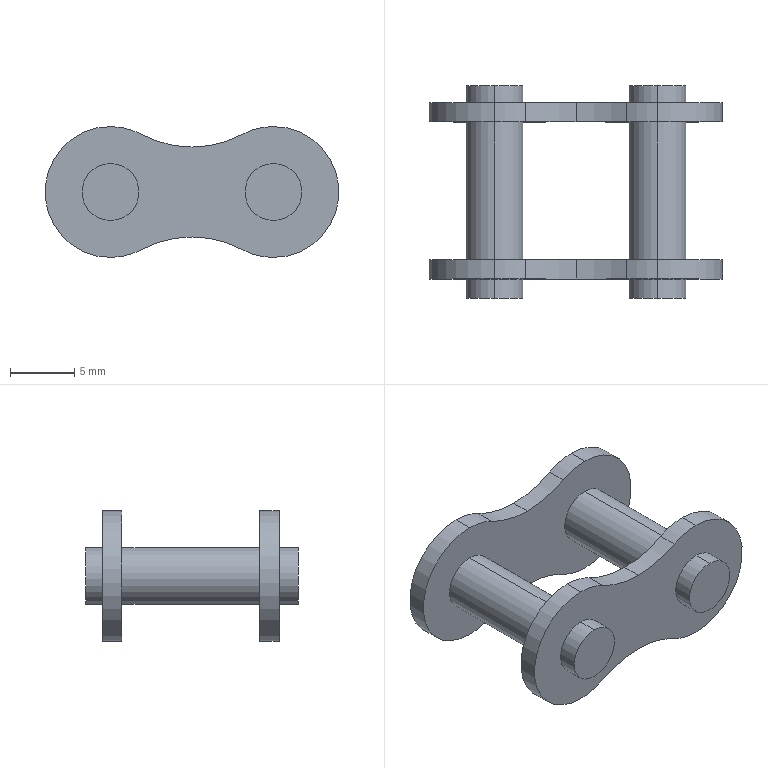Part | SolidWorks | features BaseBody 1 | 1 solid | 38 faces | box 22.9 x 16.575 x 10.2 mm | volume 988.18 mm3 | cylinder 30 | plane 8 | commonest cylinder face diameters 4.44 x12 10.2 x12 16.655 x6
STEP:
#1=CARTESIAN_POINT('',(-416.726,-324.843,-253.348));
#2=VERTEX_POINT('',#1);
#3=CARTESIAN_POINT('',(-416.726,-324.843,-257.788));
#4=VERTEX_POINT('',#3);
#5=CARTESIAN_POINT('',(-416.726,-324.843,-255.568));
#6=DIRECTION('',(-0.000000001,-1.,-0.000000001));
#7=DIRECTION('',(-0.000000001,0.000000001,-1.));
#8=AXIS2_PLACEMENT_3D('',#5,#6,#7);
#9=CIRCLE('',#8,2.22);
#10=EDGE_CURVE('',#2,#4,#9,.T.);
#11=ORIENTED_EDGE('',*,*,#10,.F.);
#12=CARTESIAN_POINT('',(-416.726,-323.343,-253.348));
#13=VERTEX_POINT('',#12);
#14=CARTESIAN_POINT('',(-416.726,-328.343,-253.348));
#15=DIRECTION('',(0.000000001,1.,0.000000001));
#16=VECTOR('',#15,1000.);
#17=LINE('',#14,#16);
#18=EDGE_CURVE('',#2,#13,#17,.T.);
#19=ORIENTED_EDGE('',*,*,#18,.T.);
#20=CARTESIAN_POINT('',(-416.726,-323.343,-257.788));
#21=VERTEX_POINT('',#20);
#22=CARTESIAN_POINT('',(-416.726,-323.343,-255.568));
#23=DIRECTION('',(0.000000001,1.,0.000000001));
#24=DIRECTION('',(-0.000000001,0.000000001,-1.));
#25=AXIS2_PLACEMENT_3D('',#22,#23,#24);
#26=CIRCLE('',#25,2.22);
#27=EDGE_CURVE('',#21,#13,#26,.T.);
#28=ORIENTED_EDGE('',*,*,#27,.F.);
#29=CARTESIAN_POINT('',(-416.726,-328.343,-257.788));
#30=DIRECTION('',(0.000000001,1.,0.000000001));
#31=VECTOR('',#30,1000.);
#32=LINE('',#29,#31);
#33=EDGE_CURVE('',#4,#21,#32,.T.);
#34=ORIENTED_EDGE('',*,*,#33,.F.);
#35=EDGE_LOOP('',(#11,#19,#28,#34));
#36=FACE_OUTER_BOUND('',#35,.T.);
#37=CARTESIAN_POINT('',(-416.726,-328.343,-255.568));
#38=DIRECTION('',(0.000000001,1.,0.000000001));
#39=DIRECTION('',(-0.000000001,0.000000001,-1.));
#40=AXIS2_PLACEMENT_3D('',#37,#38,#39);
#41=CYLINDRICAL_SURFACE('',#40,2.22);
#42=ADVANCED_FACE('',(#36),#41,.T.);
#43=CARTESIAN_POINT('',(-429.426,-324.843,-253.348));
#44=VERTEX_POINT('',#43);
#45=CARTESIAN_POINT('',(-429.426,-324.843,-257.788));
#46=VERTEX_POINT('',#45);
#47=CARTESIAN_POINT('',(-429.426,-324.843,-255.568));
#48=DIRECTION('',(-0.000000001,-1.,-0.000000001));
#49=DIRECTION('',(-0.000000001,0.000000001,-1.));
#50=AXIS2_PLACEMENT_3D('',#47,#48,#49);
#51=CIRCLE('',#50,2.22);
#52=EDGE_CURVE('',#44,#46,#51,.T.);
#53=ORIENTED_EDGE('',*,*,#52,.F.);
#54=CARTESIAN_POINT('',(-429.426,-323.343,-253.348));
#55=VERTEX_POINT('',#54);
#56=CARTESIAN_POINT('',(-429.426,-328.343,-253.348));
#57=DIRECTION('',(0.000000001,1.,0.000000001));
#58=VECTOR('',#57,1000.);
#59=LINE('',#56,#58);
#60=EDGE_CURVE('',#44,#55,#59,.T.);
#61=ORIENTED_EDGE('',*,*,#60,.T.);
#62=CARTESIAN_POINT('',(-429.426,-323.343,-257.788));
#63=VERTEX_POINT('',#62);
#64=CARTESIAN_POINT('',(-429.426,-323.343,-255.568));
#65=DIRECTION('',(0.000000001,1.,0.000000001));
#66=DIRECTION('',(-0.000000001,0.000000001,-1.));
#67=AXIS2_PLACEMENT_3D('',#64,#65,#66);
#68=CIRCLE('',#67,2.22);
#69=EDGE_CURVE('',#63,#55,#68,.T.);
#70=ORIENTED_EDGE('',*,*,#69,.F.);
#71=CARTESIAN_POINT('',(-429.426,-328.343,-257.788));
#72=DIRECTION('',(0.000000001,1.,0.000000001));
#73=VECTOR('',#72,1000.);
#74=LINE('',#71,#73);
#75=EDGE_CURVE('',#46,#63,#74,.T.);
#76=ORIENTED_EDGE('',*,*,#75,.F.);
#77=EDGE_LOOP('',(#53,#61,#70,#76));
#78=FACE_OUTER_BOUND('',#77,.T.);
#79=CARTESIAN_POINT('',(-429.426,-328.343,-255.568));
#80=DIRECTION('',(0.000000001,1.,0.000000001));
#81=DIRECTION('',(-0.000000001,0.000000001,-1.));
#82=AXIS2_PLACEMENT_3D('',#79,#80,#81);
#83=CYLINDRICAL_SURFACE('',#82,2.22);
#84=ADVANCED_FACE('',(#78),#83,.T.);
#85=CARTESIAN_POINT('',(-416.726,-309.593,-257.788));
#86=VERTEX_POINT('',#85);
#87=CARTESIAN_POINT('',(-416.726,-309.593,-253.348));
#88=VERTEX_POINT('',#87);
#89=CARTESIAN_POINT('',(-416.726,-309.593,-255.568));
#90=DIRECTION('',(0.000000001,1.,0.000000001));
#91=DIRECTION('',(-0.000000001,0.000000001,-1.));
#92=AXIS2_PLACEMENT_3D('',#89,#90,#91);
#93=CIRCLE('',#92,2.22);
#94=EDGE_CURVE('',#86,#88,#93,.T.);
#95=ORIENTED_EDGE('',*,*,#94,.T.);
#96=CARTESIAN_POINT('',(-416.726,-308.268,-253.348));
#97=VERTEX_POINT('',#96);
#98=CARTESIAN_POINT('',(-416.726,-328.343,-253.348));
#99=DIRECTION('',(0.000000001,1.,0.000000001));
#100=VECTOR('',#99,1000.);
#101=LINE('',#98,#100);
#102=EDGE_CURVE('',#88,#97,#101,.T.);
#103=ORIENTED_EDGE('',*,*,#102,.T.);
#104=CARTESIAN_POINT('',(-416.726,-308.268,-257.788));
#105=VERTEX_POINT('',#104);
#106=CARTESIAN_POINT('',(-416.726,-308.268,-255.568));
#107=DIRECTION('',(-0.000000001,-1.,-0.000000001));
#108=DIRECTION('',(-0.000000001,0.000000001,-1.));
#109=AXIS2_PLACEMENT_3D('',#106,#107,#108);
#110=CIRCLE('',#109,2.22);
#111=EDGE_CURVE('',#97,#105,#110,.T.);
#112=ORIENTED_EDGE('',*,*,#111,.T.);
#113=CARTESIAN_POINT('',(-416.726,-328.343,-257.788));
#114=DIRECTION('',(0.000000001,1.,0.000000001));
#115=VECTOR('',#114,1000.);
#116=LINE('',#113,#115);
#117=EDGE_CURVE('',#86,#105,#116,.T.);
#118=ORIENTED_EDGE('',*,*,#117,.F.);
#119=EDGE_LOOP('',(#95,#103,#112,#118));
#120=FACE_OUTER_BOUND('',#119,.T.);
#121=CARTESIAN_POINT('',(-416.726,-328.343,-255.568));
#122=DIRECTION('',(0.000000001,1.,0.000000001));
#123=DIRECTION('',(-0.000000001,0.000000001,-1.));
#124=AXIS2_PLACEMENT_3D('',#121,#122,#123);
#125=CYLINDRICAL_SURFACE('',#124,2.22);
#126=ADVANCED_FACE('',(#120),#125,.T.);
#127=CARTESIAN_POINT('',(-429.426,-321.843,-257.788));
#128=VERTEX_POINT('',#127);
#129=CARTESIAN_POINT('',(-429.426,-321.843,-253.348));
#130=VERTEX_POINT('',#129);
#131=CARTESIAN_POINT('',(-429.426,-321.843,-255.568));
#132=DIRECTION('',(0.000000001,1.,0.000000001));
#133=DIRECTION('',(-0.000000001,0.000000001,-1.));
#134=AXIS2_PLACEMENT_3D('',#131,#132,#133);
#135=CIRCLE('',#134,2.22);
#136=EDGE_CURVE('',#128,#130,#135,.T.);
#137=ORIENTED_EDGE('',*,*,#136,.T.);
#138=CARTESIAN_POINT('',(-429.426,-311.093,-253.348));
#139=VERTEX_POINT('',#138);
#140=CARTESIAN_POINT('',(-429.426,-328.343,-253.348));
#141=DIRECTION('',(0.000000001,1.,0.000000001));
#142=VECTOR('',#141,1000.);
#143=LINE('',#140,#142);
#144=EDGE_CURVE('',#130,#139,#143,.T.);
#145=ORIENTED_EDGE('',*,*,#144,.T.);
#146=CARTESIAN_POINT('',(-429.426,-311.093,-257.788));
#147=VERTEX_POINT('',#146);
#148=CARTESIAN_POINT('',(-429.426,-311.093,-255.568));
#149=DIRECTION('',(0.000000001,1.,0.000000001));
#150=DIRECTION('',(1.,-0.000000001,-0.000000001));
#151=AXIS2_PLACEMENT_3D('',#148,#149,#150);
#152=CIRCLE('',#151,2.22);
#153=EDGE_CURVE('',#147,#139,#152,.T.);
#154=ORIENTED_EDGE('',*,*,#153,.F.);
#155=CARTESIAN_POINT('',(-429.426,-328.343,-257.788));
#156=DIRECTION('',(0.000000001,1.,0.000000001));
#157=VECTOR('',#156,1000.);
#158=LINE('',#155,#157);
#159=EDGE_CURVE('',#128,#147,#158,.T.);
#160=ORIENTED_EDGE('',*,*,#159,.F.);
#161=EDGE_LOOP('',(#137,#145,#154,#160));
#162=FACE_OUTER_BOUND('',#161,.T.);
#163=CARTESIAN_POINT('',(-429.426,-328.343,-255.568));
#164=DIRECTION('',(0.000000001,1.,0.000000001));
#165=DIRECTION('',(-0.000000001,0.000000001,-1.));
#166=AXIS2_PLACEMENT_3D('',#163,#164,#165);
#167=CYLINDRICAL_SURFACE('',#166,2.22);
#168=ADVANCED_FACE('',(#162),#167,.T.);
#169=CARTESIAN_POINT('',(-429.426,-309.593,-253.348));
#170=VERTEX_POINT('',#169);
#171=CARTESIAN_POINT('',(-429.426,-309.593,-257.788));
#172=VERTEX_POINT('',#171);
#173=CARTESIAN_POINT('',(-429.426,-309.593,-255.568));
#174=DIRECTION('',(-0.000000001,-1.,-0.000000001));
#175=DIRECTION('',(-0.000000001,0.000000001,-1.));
#176=AXIS2_PLACEMENT_3D('',#173,#174,#175);
#177=CIRCLE('',#176,2.22);
#178=EDGE_CURVE('',#170,#172,#177,.T.);
#179=ORIENTED_EDGE('',*,*,#178,.F.);
#180=CARTESIAN_POINT('',(-429.426,-308.268,-253.348));
#181=VERTEX_POINT('',#180);
#182=CARTESIAN_POINT('',(-429.426,-328.343,-253.348));
#183=DIRECTION('',(0.000000001,1.,0.000000001));
#184=VECTOR('',#183,1000.);
#185=LINE('',#182,#184);
#186=EDGE_CURVE('',#170,#181,#185,.T.);
#187=ORIENTED_EDGE('',*,*,#186,.T.);
#188=CARTESIAN_POINT('',(-429.426,-308.268,-257.788));
#189=VERTEX_POINT('',#188);
#190=CARTESIAN_POINT('',(-429.426,-308.268,-255.568));
#191=DIRECTION('',(-0.000000001,-1.,-0.000000001));
#192=DIRECTION('',(-0.000000001,0.000000001,-1.));
#193=AXIS2_PLACEMENT_3D('',#190,#191,#192);
#194=CIRCLE('',#193,2.22);
#195=EDGE_CURVE('',#181,#189,#194,.T.);
#196=ORIENTED_EDGE('',*,*,#195,.T.);
#197=CARTESIAN_POINT('',(-429.426,-328.343,-257.788));
#198=DIRECTION('',(0.000000001,1.,0.000000001));
#199=VECTOR('',#198,1000.);
#200=LINE('',#197,#199);
#201=EDGE_CURVE('',#172,#189,#200,.T.);
#202=ORIENTED_EDGE('',*,*,#201,.F.);
#203=EDGE_LOOP('',(#179,#187,#196,#202));
#204=FACE_OUTER_BOUND('',#203,.T.);
#205=CARTESIAN_POINT('',(-429.426,-328.343,-255.568));
#206=DIRECTION('',(0.000000001,1.,0.000000001));
#207=DIRECTION('',(-0.000000001,0.000000001,-1.));
#208=AXIS2_PLACEMENT_3D('',#205,#206,#207);
#209=CYLINDRICAL_SURFACE('',#208,2.22);
#210=ADVANCED_FACE('',(#204),#209,.T.);
#211=CARTESIAN_POINT('',(-423.076,-311.093,-252.065));
#212=VERTEX_POINT('',#211);
#213=CARTESIAN_POINT('',(-427.014,-311.093,-251.075));
#214=VERTEX_POINT('',#213);
#215=CARTESIAN_POINT('',(-423.076,-311.093,-243.737));
#216=DIRECTION('',(0.000000001,1.,0.000000001));
#217=DIRECTION('',(1.,-0.000000001,-0.000000001));
#218=AXIS2_PLACEMENT_3D('',#215,#216,#217);
#219=CIRCLE('',#218,8.327);
#220=EDGE_CURVE('',#212,#214,#219,.T.);
#221=ORIENTED_EDGE('',*,*,#220,.F.);
#222=CARTESIAN_POINT('',(-423.076,-309.593,-252.065));
#223=VERTEX_POINT('',#222);
#224=CARTESIAN_POINT('',(-423.076,-311.093,-252.065));
#225=DIRECTION('',(0.000000001,1.,0.000000001));
#226=VECTOR('',#225,1000.);
#227=LINE('',#224,#226);
#228=EDGE_CURVE('',#212,#223,#227,.T.);
#229=ORIENTED_EDGE('',*,*,#228,.T.);
#230=CARTESIAN_POINT('',(-427.014,-309.593,-251.075));
#231=VERTEX_POINT('',#230);
#232=CARTESIAN_POINT('',(-423.076,-309.593,-243.737));
#233=DIRECTION('',(0.000000001,1.,0.000000001));
#234=DIRECTION('',(1.,-0.000000001,-0.000000001));
#235=AXIS2_PLACEMENT_3D('',#232,#233,#234);
#236=CIRCLE('',#235,8.327);
#237=EDGE_CURVE('',#223,#231,#236,.T.);
#238=ORIENTED_EDGE('',*,*,#237,.T.);
#239=CARTESIAN_POINT('',(-427.014,-311.093,-251.075));
#240=DIRECTION('',(0.000000001,1.,0.000000001));
#241=VECTOR('',#240,1000.);
#242=LINE('',#239,#241);
#243=EDGE_CURVE('',#214,#231,#242,.T.);
#244=ORIENTED_EDGE('',*,*,#243,.F.);
#245=EDGE_LOOP('',(#221,#229,#238,#244));
#246=FACE_OUTER_BOUND('',#245,.T.);
#247=CARTESIAN_POINT('',(-423.076,-311.093,-243.737));
#248=DIRECTION('',(0.000000001,1.,0.000000001));
#249=DIRECTION('',(-0.000000001,0.000000001,-1.));
#250=AXIS2_PLACEMENT_3D('',#247,#248,#249);
#251=CYLINDRICAL_SURFACE('',#250,8.327);
#252=ADVANCED_FACE('',(#246),#251,.F.);
#253=CARTESIAN_POINT('',(-416.726,-311.093,-250.468));
#254=VERTEX_POINT('',#253);
#255=CARTESIAN_POINT('',(-419.115,-311.093,-251.063));
#256=VERTEX_POINT('',#255);
#257=CARTESIAN_POINT('',(-416.726,-311.093,-255.568));
#258=DIRECTION('',(-0.000000001,-1.,-0.000000001));
#259=DIRECTION('',(1.,-0.000000001,-0.000000001));
#260=AXIS2_PLACEMENT_3D('',#257,#258,#259);
#261=CIRCLE('',#260,5.1);
#262=EDGE_CURVE('',#254,#256,#261,.T.);
#263=ORIENTED_EDGE('',*,*,#262,.F.);
#264=CARTESIAN_POINT('',(-416.726,-309.593,-250.468));
#265=VERTEX_POINT('',#264);
#266=CARTESIAN_POINT('',(-416.726,-311.093,-250.468));
#267=DIRECTION('',(0.000000001,1.,0.000000001));
#268=VECTOR('',#267,1000.);
#269=LINE('',#266,#268);
#270=EDGE_CURVE('',#254,#265,#269,.T.);
#271=ORIENTED_EDGE('',*,*,#270,.T.);
#272=CARTESIAN_POINT('',(-419.115,-309.593,-251.063));
#273=VERTEX_POINT('',#272);
#274=CARTESIAN_POINT('',(-416.726,-309.593,-255.568));
#275=DIRECTION('',(-0.000000001,-1.,-0.000000001));
#276=DIRECTION('',(1.,-0.000000001,-0.000000001));
#277=AXIS2_PLACEMENT_3D('',#274,#275,#276);
#278=CIRCLE('',#277,5.1);
#279=EDGE_CURVE('',#265,#273,#278,.T.);
#280=ORIENTED_EDGE('',*,*,#279,.T.);
#281=CARTESIAN_POINT('',(-419.115,-311.093,-251.063));
#282=DIRECTION('',(0.000000001,1.,0.000000001));
#283=VECTOR('',#282,1000.);
#284=LINE('',#281,#283);
#285=EDGE_CURVE('',#256,#273,#284,.T.);
#286=ORIENTED_EDGE('',*,*,#285,.F.);
#287=EDGE_LOOP('',(#263,#271,#280,#286));
#288=FACE_OUTER_BOUND('',#287,.T.);
#289=CARTESIAN_POINT('',(-416.726,-311.093,-255.568));
#290=DIRECTION('',(0.000000001,1.,0.000000001));
#291=DIRECTION('',(-0.000000001,0.000000001,-1.));
#292=AXIS2_PLACEMENT_3D('',#289,#290,#291);
#293=CYLINDRICAL_SURFACE('',#292,5.1);
#294=ADVANCED_FACE('',(#288),#293,.T.);
#295=ORIENTED_EDGE('',*,*,#270,.F.);
#296=CARTESIAN_POINT('',(-416.726,-311.093,-260.668));
#297=VERTEX_POINT('',#296);
#298=CARTESIAN_POINT('',(-416.726,-311.093,-255.568));
#299=DIRECTION('',(-0.000000001,-1.,-0.000000001));
#300=DIRECTION('',(1.,-0.000000001,-0.000000001));
#301=AXIS2_PLACEMENT_3D('',#298,#299,#300);
#302=CIRCLE('',#301,5.1);
#303=EDGE_CURVE('',#297,#254,#302,.T.);
#304=ORIENTED_EDGE('',*,*,#303,.F.);
#305=CARTESIAN_POINT('',(-416.726,-309.593,-260.668));
#306=VERTEX_POINT('',#305);
#307=CARTESIAN_POINT('',(-416.726,-311.093,-260.668));
#308=DIRECTION('',(0.000000001,1.,0.000000001));
#309=VECTOR('',#308,1000.);
#310=LINE('',#307,#309);
#311=EDGE_CURVE('',#297,#306,#310,.T.);
#312=ORIENTED_EDGE('',*,*,#311,.T.);
#313=CARTESIAN_POINT('',(-416.726,-309.593,-255.568));
#314=DIRECTION('',(-0.000000001,-1.,-0.000000001));
#315=DIRECTION('',(1.,-0.000000001,-0.000000001));
#316=AXIS2_PLACEMENT_3D('',#313,#314,#315);
#317=CIRCLE('',#316,5.1);
#318=EDGE_CURVE('',#306,#265,#317,.T.);
#319=ORIENTED_EDGE('',*,*,#318,.T.);
#320=EDGE_LOOP('',(#295,#304,#312,#319));
#321=FACE_OUTER_BOUND('',#320,.T.);
#322=CARTESIAN_POINT('',(-416.726,-311.093,-255.568));
#323=DIRECTION('',(0.000000001,1.,0.000000001));
#324=DIRECTION('',(-0.000000001,0.000000001,-1.));
#325=AXIS2_PLACEMENT_3D('',#322,#323,#324);
#326=CYLINDRICAL_SURFACE('',#325,5.1);
#327=ADVANCED_FACE('',(#321),#326,.T.);
#328=CARTESIAN_POINT('',(-429.426,-311.093,-250.468));
#329=VERTEX_POINT('',#328);
#330=CARTESIAN_POINT('',(-429.426,-311.093,-260.668));
#331=VERTEX_POINT('',#330);
#332=CARTESIAN_POINT('',(-429.426,-311.093,-255.568));
#333=DIRECTION('',(-0.000000001,-1.,-0.000000001));
#334=DIRECTION('',(1.,-0.000000001,-0.000000001));
#335=AXIS2_PLACEMENT_3D('',#332,#333,#334);
#336=CIRCLE('',#335,5.1);
#337=EDGE_CURVE('',#329,#331,#336,.T.);
#338=ORIENTED_EDGE('',*,*,#337,.F.);
#339=CARTESIAN_POINT('',(-429.426,-309.593,-250.468));
#340=VERTEX_POINT('',#339);
#341=CARTESIAN_POINT('',(-429.426,-311.093,-250.468));
#342=DIRECTION('',(0.000000001,1.,0.000000001));
#343=VECTOR('',#342,1000.);
#344=LINE('',#341,#343);
#345=EDGE_CURVE('',#329,#340,#344,.T.);
#346=ORIENTED_EDGE('',*,*,#345,.T.);
#347=CARTESIAN_POINT('',(-429.426,-309.593,-260.668));
#348=VERTEX_POINT('',#347);
#349=CARTESIAN_POINT('',(-429.426,-309.593,-255.568));
#350=DIRECTION('',(-0.000000001,-1.,-0.000000001));
#351=DIRECTION('',(1.,-0.000000001,-0.000000001));
#352=AXIS2_PLACEMENT_3D('',#349,#350,#351);
#353=CIRCLE('',#352,5.1);
#354=EDGE_CURVE('',#340,#348,#353,.T.);
#355=ORIENTED_EDGE('',*,*,#354,.T.);
#356=CARTESIAN_POINT('',(-429.426,-311.093,-260.668));
#357=DIRECTION('',(0.000000001,1.,0.000000001));
#358=VECTOR('',#357,1000.);
#359=LINE('',#356,#358);
#360=EDGE_CURVE('',#331,#348,#359,.T.);
#361=ORIENTED_EDGE('',*,*,#360,.F.);
#362=EDGE_LOOP('',(#338,#346,#355,#361));
#363=FACE_OUTER_BOUND('',#362,.T.);
#364=CARTESIAN_POINT('',(-429.426,-311.093,-255.568));
#365=DIRECTION('',(0.000000001,1.,0.000000001));
#366=DIRECTION('',(-0.000000001,0.000000001,-1.));
#367=AXIS2_PLACEMENT_3D('',#364,#365,#366);
#368=CYLINDRICAL_SURFACE('',#367,5.1);
#369=ADVANCED_FACE('',(#363),#368,.T.);
#370=CARTESIAN_POINT('',(-427.014,-311.093,-260.062));
#371=VERTEX_POINT('',#370);
#372=CARTESIAN_POINT('',(-429.426,-311.093,-255.568));
#373=DIRECTION('',(-0.000000001,-1.,-0.000000001));
#374=DIRECTION('',(1.,-0.000000001,-0.000000001));
#375=AXIS2_PLACEMENT_3D('',#372,#373,#374);
#376=CIRCLE('',#375,5.1);
#377=EDGE_CURVE('',#331,#371,#376,.T.);
#378=ORIENTED_EDGE('',*,*,#377,.F.);
#379=ORIENTED_EDGE('',*,*,#360,.T.);
#380=CARTESIAN_POINT('',(-427.014,-309.593,-260.062));
#381=VERTEX_POINT('',#380);
#382=CARTESIAN_POINT('',(-429.426,-309.593,-255.568));
#383=DIRECTION('',(-0.000000001,-1.,-0.000000001));
#384=DIRECTION('',(1.,-0.000000001,-0.000000001));
#385=AXIS2_PLACEMENT_3D('',#382,#383,#384);
#386=CIRCLE('',#385,5.1);
#387=EDGE_CURVE('',#348,#381,#386,.T.);
#388=ORIENTED_EDGE('',*,*,#387,.T.);
#389=CARTESIAN_POINT('',(-427.014,-311.093,-260.062));
#390=DIRECTION('',(0.000000001,1.,0.000000001));
#391=VECTOR('',#390,1000.);
#392=LINE('',#389,#391);
#393=EDGE_CURVE('',#371,#381,#392,.T.);
#394=ORIENTED_EDGE('',*,*,#393,.F.);
#395=EDGE_LOOP('',(#378,#379,#388,#394));
#396=FACE_OUTER_BOUND('',#395,.T.);
#397=CARTESIAN_POINT('',(-429.426,-311.093,-255.568));
#398=DIRECTION('',(0.000000001,1.,0.000000001));
#399=DIRECTION('',(-0.000000001,0.000000001,-1.));
#400=AXIS2_PLACEMENT_3D('',#397,#398,#399);
#401=CYLINDRICAL_SURFACE('',#400,5.1);
#402=ADVANCED_FACE('',(#396),#401,.T.);
#403=CARTESIAN_POINT('',(-416.726,-321.843,-257.788));
#404=VERTEX_POINT('',#403);
#405=CARTESIAN_POINT('',(-416.726,-321.843,-253.348));
#406=VERTEX_POINT('',#405);
#407=CARTESIAN_POINT('',(-416.726,-321.843,-255.568));
#408=DIRECTION('',(0.000000001,1.,0.000000001));
#409=DIRECTION('',(-0.000000001,0.000000001,-1.));
#410=AXIS2_PLACEMENT_3D('',#407,#408,#409);
#411=CIRCLE('',#410,2.22);
#412=EDGE_CURVE('',#404,#406,#411,.T.);
#413=ORIENTED_EDGE('',*,*,#412,.T.);
#414=CARTESIAN_POINT('',(-416.726,-311.093,-253.348));
#415=VERTEX_POINT('',#414);
#416=CARTESIAN_POINT('',(-416.726,-328.343,-253.348));
#417=DIRECTION('',(0.000000001,1.,0.000000001));
#418=VECTOR('',#417,1000.);
#419=LINE('',#416,#418);
#420=EDGE_CURVE('',#406,#415,#419,.T.);
#421=ORIENTED_EDGE('',*,*,#420,.T.);
#422=CARTESIAN_POINT('',(-416.726,-311.093,-257.788));
#423=VERTEX_POINT('',#422);
#424=CARTESIAN_POINT('',(-416.726,-311.093,-255.568));
#425=DIRECTION('',(0.000000001,1.,0.000000001));
#426=DIRECTION('',(1.,-0.000000001,-0.000000001));
#427=AXIS2_PLACEMENT_3D('',#424,#425,#426);
#428=CIRCLE('',#427,2.22);
#429=EDGE_CURVE('',#423,#415,#428,.T.);
#430=ORIENTED_EDGE('',*,*,#429,.F.);
#431=CARTESIAN_POINT('',(-416.726,-328.343,-257.788));
#432=DIRECTION('',(0.000000001,1.,0.000000001));
#433=VECTOR('',#432,1000.);
#434=LINE('',#431,#433);
#435=EDGE_CURVE('',#404,#423,#434,.T.);
#436=ORIENTED_EDGE('',*,*,#435,.F.);
#437=EDGE_LOOP('',(#413,#421,#430,#436));
#438=FACE_OUTER_BOUND('',#437,.T.);
#439=CARTESIAN_POINT('',(-416.726,-328.343,-255.568));
#440=DIRECTION('',(0.000000001,1.,0.000000001));
#441=DIRECTION('',(-0.000000001,0.000000001,-1.));
#442=AXIS2_PLACEMENT_3D('',#439,#440,#441);
#443=CYLINDRICAL_SURFACE('',#442,2.22);
#444=ADVANCED_FACE('',(#438),#443,.T.);
#445=CARTESIAN_POINT('',(-429.426,-323.343,-250.468));
#446=VERTEX_POINT('',#445);
#447=CARTESIAN_POINT('',(-429.426,-323.343,-260.668));
#448=VERTEX_POINT('',#447);
#449=CARTESIAN_POINT('',(-429.426,-323.343,-255.568));
#450=DIRECTION('',(-0.000000001,-1.,-0.000000001));
#451=DIRECTION('',(-0.000000001,0.000000001,-1.));
#452=AXIS2_PLACEMENT_3D('',#449,#450,#451);
#453=CIRCLE('',#452,5.1);
#454=EDGE_CURVE('',#446,#448,#453,.T.);
#455=ORIENTED_EDGE('',*,*,#454,.F.);
#456=CARTESIAN_POINT('',(-429.426,-321.843,-250.468));
#457=VERTEX_POINT('',#456);
#458=CARTESIAN_POINT('',(-429.426,-324.843,-250.468));
#459=DIRECTION('',(0.000000001,1.,0.000000001));
#460=VECTOR('',#459,1000.);
#461=LINE('',#458,#460);
#462=EDGE_CURVE('',#446,#457,#461,.T.);
#463=ORIENTED_EDGE('',*,*,#462,.T.);
#464=CARTESIAN_POINT('',(-429.426,-321.843,-260.668));
#465=VERTEX_POINT('',#464);
#466=CARTESIAN_POINT('',(-429.426,-321.843,-255.568));
#467=DIRECTION('',(-0.000000001,-1.,-0.000000001));
#468=DIRECTION('',(1.,-0.000000001,-0.000000001));
#469=AXIS2_PLACEMENT_3D('',#466,#467,#468);
#470=CIRCLE('',#469,5.1);
#471=EDGE_CURVE('',#457,#465,#470,.T.);
#472=ORIENTED_EDGE('',*,*,#471,.T.);
#473=CARTESIAN_POINT('',(-429.426,-324.843,-260.668));
#474=DIRECTION('',(0.000000001,1.,0.000000001));
#475=VECTOR('',#474,1000.);
#476=LINE('',#473,#475);
#477=EDGE_CURVE('',#448,#465,#476,.T.);
#478=ORIENTED_EDGE('',*,*,#477,.F.);
#479=EDGE_LOOP('',(#455,#463,#472,#478));
#480=FACE_OUTER_BOUND('',#479,.T.);
#481=CARTESIAN_POINT('',(-429.426,-324.843,-255.568));
#482=DIRECTION('',(0.000000001,1.,0.000000001));
#483=DIRECTION('',(-0.000000001,0.000000001,-1.));
#484=AXIS2_PLACEMENT_3D('',#481,#482,#483);
#485=CYLINDRICAL_SURFACE('',#484,5.1);
#486=ADVANCED_FACE('',(#480),#485,.T.);
#487=CARTESIAN_POINT('',(-427.014,-323.343,-260.062));
#488=VERTEX_POINT('',#487);
#489=CARTESIAN_POINT('',(-429.426,-323.343,-255.568));
#490=DIRECTION('',(-0.000000001,-1.,-0.000000001));
#491=DIRECTION('',(-0.000000001,0.000000001,-1.));
#492=AXIS2_PLACEMENT_3D('',#489,#490,#491);
#493=CIRCLE('',#492,5.1);
#494=EDGE_CURVE('',#448,#488,#493,.T.);
#495=ORIENTED_EDGE('',*,*,#494,.F.);
#496=ORIENTED_EDGE('',*,*,#477,.T.);
#497=CARTESIAN_POINT('',(-427.014,-321.843,-260.062));
#498=VERTEX_POINT('',#497);
#499=CARTESIAN_POINT('',(-429.426,-321.843,-255.568));
#500=DIRECTION('',(-0.000000001,-1.,-0.000000001));
#501=DIRECTION('',(1.,-0.000000001,-0.000000001));
#502=AXIS2_PLACEMENT_3D('',#499,#500,#501);
#503=CIRCLE('',#502,5.1);
#504=EDGE_CURVE('',#465,#498,#503,.T.);
#505=ORIENTED_EDGE('',*,*,#504,.T.);
#506=CARTESIAN_POINT('',(-427.014,-324.843,-260.062));
#507=DIRECTION('',(0.000000001,1.,0.000000001));
#508=VECTOR('',#507,1000.);
#509=LINE('',#506,#508);
#510=EDGE_CURVE('',#488,#498,#509,.T.);
#511=ORIENTED_EDGE('',*,*,#510,.F.);
#512=EDGE_LOOP('',(#495,#496,#505,#511));
#513=FACE_OUTER_BOUND('',#512,.T.);
#514=CARTESIAN_POINT('',(-429.426,-324.843,-255.568));
#515=DIRECTION('',(0.000000001,1.,0.000000001));
#516=DIRECTION('',(-0.000000001,0.000000001,-1.));
#517=AXIS2_PLACEMENT_3D('',#514,#515,#516);
#518=CYLINDRICAL_SURFACE('',#517,5.1);
#519=ADVANCED_FACE('',(#513),#518,.T.);
#520=CARTESIAN_POINT('',(-416.726,-323.343,-250.468));
#521=VERTEX_POINT('',#520);
#522=CARTESIAN_POINT('',(-419.115,-323.343,-251.063));
#523=VERTEX_POINT('',#522);
#524=CARTESIAN_POINT('',(-416.726,-323.343,-255.568));
#525=DIRECTION('',(-0.000000001,-1.,-0.000000001));
#526=DIRECTION('',(-0.000000001,0.000000001,-1.));
#527=AXIS2_PLACEMENT_3D('',#524,#525,#526);
#528=CIRCLE('',#527,5.1);
#529=EDGE_CURVE('',#521,#523,#528,.T.);
#530=ORIENTED_EDGE('',*,*,#529,.F.);
#531=CARTESIAN_POINT('',(-416.726,-321.843,-250.468));
#532=VERTEX_POINT('',#531);
#533=CARTESIAN_POINT('',(-416.726,-324.843,-250.468));
#534=DIRECTION('',(0.000000001,1.,0.000000001));
#535=VECTOR('',#534,1000.);
#536=LINE('',#533,#535);
#537=EDGE_CURVE('',#521,#532,#536,.T.);
#538=ORIENTED_EDGE('',*,*,#537,.T.);
#539=CARTESIAN_POINT('',(-419.115,-321.843,-251.063));
#540=VERTEX_POINT('',#539);
#541=CARTESIAN_POINT('',(-416.726,-321.843,-255.568));
#542=DIRECTION('',(-0.000000001,-1.,-0.000000001));
#543=DIRECTION('',(1.,-0.000000001,-0.000000001));
#544=AXIS2_PLACEMENT_3D('',#541,#542,#543);
#545=CIRCLE('',#544,5.1);
#546=EDGE_CURVE('',#532,#540,#545,.T.);
#547=ORIENTED_EDGE('',*,*,#546,.T.);
#548=CARTESIAN_POINT('',(-419.115,-324.843,-251.063));
#549=DIRECTION('',(0.000000001,1.,0.000000001));
#550=VECTOR('',#549,1000.);
#551=LINE('',#548,#550);
#552=EDGE_CURVE('',#523,#540,#551,.T.);
#553=ORIENTED_EDGE('',*,*,#552,.F.);
#554=EDGE_LOOP('',(#530,#538,#547,#553));
#555=FACE_OUTER_BOUND('',#554,.T.);
#556=CARTESIAN_POINT('',(-416.726,-324.843,-255.568));
#557=DIRECTION('',(0.000000001,1.,0.000000001));
#558=DIRECTION('',(-0.000000001,0.000000001,-1.));
#559=AXIS2_PLACEMENT_3D('',#556,#557,#558);
#560=CYLINDRICAL_SURFACE('',#559,5.1);
#561=ADVANCED_FACE('',(#555),#560,.T.);
#562=ORIENTED_EDGE('',*,*,#537,.F.);
#563=CARTESIAN_POINT('',(-416.726,-323.343,-260.668));
#564=VERTEX_POINT('',#563);
#565=CARTESIAN_POINT('',(-416.726,-323.343,-255.568));
#566=DIRECTION('',(-0.000000001,-1.,-0.000000001));
#567=DIRECTION('',(-0.000000001,0.000000001,-1.));
#568=AXIS2_PLACEMENT_3D('',#565,#566,#567);
#569=CIRCLE('',#568,5.1);
#570=EDGE_CURVE('',#564,#521,#569,.T.);
#571=ORIENTED_EDGE('',*,*,#570,.F.);
#572=CARTESIAN_POINT('',(-416.726,-321.843,-260.668));
#573=VERTEX_POINT('',#572);
#574=CARTESIAN_POINT('',(-416.726,-324.843,-260.668));
#575=DIRECTION('',(0.000000001,1.,0.000000001));
#576=VECTOR('',#575,1000.);
#577=LINE('',#574,#576);
#578=EDGE_CURVE('',#564,#573,#577,.T.);
#579=ORIENTED_EDGE('',*,*,#578,.T.);
#580=CARTESIAN_POINT('',(-416.726,-321.843,-255.568));
#581=DIRECTION('',(-0.000000001,-1.,-0.000000001));
#582=DIRECTION('',(1.,-0.000000001,-0.000000001));
#583=AXIS2_PLACEMENT_3D('',#580,#581,#582);
#584=CIRCLE('',#583,5.1);
#585=EDGE_CURVE('',#573,#532,#584,.T.);
#586=ORIENTED_EDGE('',*,*,#585,.T.);
#587=EDGE_LOOP('',(#562,#571,#579,#586));
#588=FACE_OUTER_BOUND('',#587,.T.);
#589=CARTESIAN_POINT('',(-416.726,-324.843,-255.568));
#590=DIRECTION('',(0.000000001,1.,0.000000001));
#591=DIRECTION('',(-0.000000001,0.000000001,-1.));
#592=AXIS2_PLACEMENT_3D('',#589,#590,#591);
#593=CYLINDRICAL_SURFACE('',#592,5.1);
#594=ADVANCED_FACE('',(#588),#593,.T.);
#595=CARTESIAN_POINT('',(-423.076,-323.343,-252.065));
#596=VERTEX_POINT('',#595);
#597=CARTESIAN_POINT('',(-427.014,-323.343,-251.075));
#598=VERTEX_POINT('',#597);
#599=CARTESIAN_POINT('',(-423.076,-323.343,-243.737));
#600=DIRECTION('',(0.000000001,1.,0.000000001));
#601=DIRECTION('',(-0.000000001,0.000000001,-1.));
#602=AXIS2_PLACEMENT_3D('',#599,#600,#601);
#603=CIRCLE('',#602,8.327);
#604=EDGE_CURVE('',#596,#598,#603,.T.);
#605=ORIENTED_EDGE('',*,*,#604,.F.);
#606=CARTESIAN_POINT('',(-423.076,-321.843,-252.065));
#607=VERTEX_POINT('',#606);
#608=CARTESIAN_POINT('',(-423.076,-324.843,-252.065));
#609=DIRECTION('',(0.000000001,1.,0.000000001));
#610=VECTOR('',#609,1000.);
#611=LINE('',#608,#610);
#612=EDGE_CURVE('',#596,#607,#611,.T.);
#613=ORIENTED_EDGE('',*,*,#612,.T.);
#614=CARTESIAN_POINT('',(-427.014,-321.843,-251.075));
#615=VERTEX_POINT('',#614);
#616=CARTESIAN_POINT('',(-423.076,-321.843,-243.737));
#617=DIRECTION('',(0.000000001,1.,0.000000001));
#618=DIRECTION('',(1.,-0.000000001,-0.000000001));
#619=AXIS2_PLACEMENT_3D('',#616,#617,#618);
#620=CIRCLE('',#619,8.327);
#621=EDGE_CURVE('',#607,#615,#620,.T.);
#622=ORIENTED_EDGE('',*,*,#621,.T.);
#623=CARTESIAN_POINT('',(-427.014,-324.843,-251.075));
#624=DIRECTION('',(0.000000001,1.,0.000000001));
#625=VECTOR('',#624,1000.);
#626=LINE('',#623,#625);
#627=EDGE_CURVE('',#598,#615,#626,.T.);
#628=ORIENTED_EDGE('',*,*,#627,.F.);
#629=EDGE_LOOP('',(#605,#613,#622,#628));
#630=FACE_OUTER_BOUND('',#629,.T.);
#631=CARTESIAN_POINT('',(-423.076,-324.843,-243.737));
#632=DIRECTION('',(0.000000001,1.,0.000000001));
#633=DIRECTION('',(-0.000000001,0.000000001,-1.));
#634=AXIS2_PLACEMENT_3D('',#631,#632,#633);
#635=CYLINDRICAL_SURFACE('',#634,8.327);
#636=ADVANCED_FACE('',(#630),#635,.F.);
#637=ORIENTED_EDGE('',*,*,#612,.F.);
#638=CARTESIAN_POINT('',(-423.076,-323.343,-243.737));
#639=DIRECTION('',(0.000000001,1.,0.000000001));
#640=DIRECTION('',(-0.000000001,0.000000001,-1.));
#641=AXIS2_PLACEMENT_3D('',#638,#639,#640);
#642=CIRCLE('',#641,8.327);
#643=EDGE_CURVE('',#523,#596,#642,.T.);
#644=ORIENTED_EDGE('',*,*,#643,.F.);
#645=ORIENTED_EDGE('',*,*,#552,.T.);
#646=CARTESIAN_POINT('',(-423.076,-321.843,-243.737));
#647=DIRECTION('',(0.000000001,1.,0.000000001));
#648=DIRECTION('',(1.,-0.000000001,-0.000000001));
#649=AXIS2_PLACEMENT_3D('',#646,#647,#648);
#650=CIRCLE('',#649,8.327);
#651=EDGE_CURVE('',#540,#607,#650,.T.);
#652=ORIENTED_EDGE('',*,*,#651,.T.);
#653=EDGE_LOOP('',(#637,#644,#645,#652));
#654=FACE_OUTER_BOUND('',#653,.T.);
#655=CARTESIAN_POINT('',(-423.076,-324.843,-243.737));
#656=DIRECTION('',(0.000000001,1.,0.000000001));
#657=DIRECTION('',(-0.000000001,0.000000001,-1.));
#658=AXIS2_PLACEMENT_3D('',#655,#656,#657);
#659=CYLINDRICAL_SURFACE('',#658,8.327);
#660=ADVANCED_FACE('',(#654),#659,.F.);
#661=ORIENTED_EDGE('',*,*,#578,.F.);
#662=CARTESIAN_POINT('',(-419.115,-323.343,-260.074));
#663=VERTEX_POINT('',#662);
#664=CARTESIAN_POINT('',(-416.726,-323.343,-255.568));
#665=DIRECTION('',(-0.000000001,-1.,-0.000000001));
#666=DIRECTION('',(-0.000000001,0.000000001,-1.));
#667=AXIS2_PLACEMENT_3D('',#664,#665,#666);
#668=CIRCLE('',#667,5.1);
#669=EDGE_CURVE('',#663,#564,#668,.T.);
#670=ORIENTED_EDGE('',*,*,#669,.F.);
#671=CARTESIAN_POINT('',(-419.115,-321.843,-260.074));
#672=VERTEX_POINT('',#671);
#673=CARTESIAN_POINT('',(-419.115,-324.843,-260.074));
#674=DIRECTION('',(0.000000001,1.,0.000000001));
#675=VECTOR('',#674,1000.);
#676=LINE('',#673,#675);
#677=EDGE_CURVE('',#663,#672,#676,.T.);
#678=ORIENTED_EDGE('',*,*,#677,.T.);
#679=CARTESIAN_POINT('',(-416.726,-321.843,-255.568));
#680=DIRECTION('',(-0.000000001,-1.,-0.000000001));
#681=DIRECTION('',(1.,-0.000000001,-0.000000001));
#682=AXIS2_PLACEMENT_3D('',#679,#680,#681);
#683=CIRCLE('',#682,5.1);
#684=EDGE_CURVE('',#672,#573,#683,.T.);
#685=ORIENTED_EDGE('',*,*,#684,.T.);
#686=EDGE_LOOP('',(#661,#670,#678,#685));
#687=FACE_OUTER_BOUND('',#686,.T.);
#688=CARTESIAN_POINT('',(-416.726,-324.843,-255.568));
#689=DIRECTION('',(0.000000001,1.,0.000000001));
#690=DIRECTION('',(-0.000000001,0.000000001,-1.));
#691=AXIS2_PLACEMENT_3D('',#688,#689,#690);
#692=CYLINDRICAL_SURFACE('',#691,5.1);
#693=ADVANCED_FACE('',(#687),#692,.T.);
#694=ORIENTED_EDGE('',*,*,#510,.T.);
#695=CARTESIAN_POINT('',(-423.076,-321.843,-267.399));
#696=DIRECTION('',(0.000000001,1.,0.000000001));
#697=DIRECTION('',(1.,-0.000000001,-0.000000001));
#698=AXIS2_PLACEMENT_3D('',#695,#696,#697);
#699=CIRCLE('',#698,8.327);
#700=EDGE_CURVE('',#498,#672,#699,.T.);
#701=ORIENTED_EDGE('',*,*,#700,.T.);
#702=ORIENTED_EDGE('',*,*,#677,.F.);
#703=CARTESIAN_POINT('',(-423.076,-323.343,-267.399));
#704=DIRECTION('',(0.000000001,1.,0.000000001));
#705=DIRECTION('',(-0.000000001,0.000000001,-1.));
#706=AXIS2_PLACEMENT_3D('',#703,#704,#705);
#707=CIRCLE('',#706,8.327);
#708=EDGE_CURVE('',#488,#663,#707,.T.);
#709=ORIENTED_EDGE('',*,*,#708,.F.);
#710=EDGE_LOOP('',(#694,#701,#702,#709));
#711=FACE_OUTER_BOUND('',#710,.T.);
#712=CARTESIAN_POINT('',(-423.076,-324.843,-267.399));
#713=DIRECTION('',(0.000000001,1.,0.000000001));
#714=DIRECTION('',(-0.000000001,0.000000001,-1.));
#715=AXIS2_PLACEMENT_3D('',#712,#713,#714);
#716=CYLINDRICAL_SURFACE('',#715,8.327);
#717=ADVANCED_FACE('',(#711),#716,.F.);
#718=ORIENTED_EDGE('',*,*,#462,.F.);
#719=CARTESIAN_POINT('',(-429.426,-323.343,-255.568));
#720=DIRECTION('',(-0.000000001,-1.,-0.000000001));
#721=DIRECTION('',(-0.000000001,0.000000001,-1.));
#722=AXIS2_PLACEMENT_3D('',#719,#720,#721);
#723=CIRCLE('',#722,5.1);
#724=EDGE_CURVE('',#598,#446,#723,.T.);
#725=ORIENTED_EDGE('',*,*,#724,.F.);
#726=ORIENTED_EDGE('',*,*,#627,.T.);
#727=CARTESIAN_POINT('',(-429.426,-321.843,-255.568));
#728=DIRECTION('',(-0.000000001,-1.,-0.000000001));
#729=DIRECTION('',(1.,-0.000000001,-0.000000001));
#730=AXIS2_PLACEMENT_3D('',#727,#728,#729);
#731=CIRCLE('',#730,5.1);
#732=EDGE_CURVE('',#615,#457,#731,.T.);
#733=ORIENTED_EDGE('',*,*,#732,.T.);
#734=EDGE_LOOP('',(#718,#725,#726,#733));
#735=FACE_OUTER_BOUND('',#734,.T.);
#736=CARTESIAN_POINT('',(-429.426,-324.843,-255.568));
#737=DIRECTION('',(0.000000001,1.,0.000000001));
#738=DIRECTION('',(-0.000000001,0.000000001,-1.));
#739=AXIS2_PLACEMENT_3D('',#736,#737,#738);
#740=CYLINDRICAL_SURFACE('',#739,5.1);
#741=ADVANCED_FACE('',(#735),#740,.T.);
#742=ORIENTED_EDGE('',*,*,#136,.F.);
#743=CARTESIAN_POINT('',(-429.426,-321.843,-255.568));
#744=DIRECTION('',(0.000000001,1.,0.000000001));
#745=DIRECTION('',(-0.000000001,0.000000001,-1.));
#746=AXIS2_PLACEMENT_3D('',#743,#744,#745);
#747=CIRCLE('',#746,2.22);
#748=EDGE_CURVE('',#130,#128,#747,.T.);
#749=ORIENTED_EDGE('',*,*,#748,.F.);
#750=EDGE_LOOP('',(#742,#749));
#751=FACE_BOUND('',#750,.T.);
#752=ORIENTED_EDGE('',*,*,#412,.F.);
#753=CARTESIAN_POINT('',(-416.726,-321.843,-255.568));
#754=DIRECTION('',(0.000000001,1.,0.000000001));
#755=DIRECTION('',(-0.000000001,0.000000001,-1.));
#756=AXIS2_PLACEMENT_3D('',#753,#754,#755);
#757=CIRCLE('',#756,2.22);
#758=EDGE_CURVE('',#406,#404,#757,.T.);
#759=ORIENTED_EDGE('',*,*,#758,.F.);
#760=EDGE_LOOP('',(#752,#759));
#761=FACE_BOUND('',#760,.T.);
#762=ORIENTED_EDGE('',*,*,#732,.F.);
#763=ORIENTED_EDGE('',*,*,#621,.F.);
#764=ORIENTED_EDGE('',*,*,#651,.F.);
#765=ORIENTED_EDGE('',*,*,#546,.F.);
#766=ORIENTED_EDGE('',*,*,#585,.F.);
#767=ORIENTED_EDGE('',*,*,#684,.F.);
#768=ORIENTED_EDGE('',*,*,#700,.F.);
#769=ORIENTED_EDGE('',*,*,#504,.F.);
#770=ORIENTED_EDGE('',*,*,#471,.F.);
#771=EDGE_LOOP('',(#762,#763,#764,#765,#766,#767,#768,#769,#770));
#772=FACE_OUTER_BOUND('',#771,.T.);
#773=CARTESIAN_POINT('',(-426.251,-321.843,-261.484));
#774=DIRECTION('',(0.000000001,1.,0.000000001));
#775=DIRECTION('',(-0.000000001,0.000000001,-1.));
#776=AXIS2_PLACEMENT_3D('',#773,#774,#775);
#777=PLANE('',#776);
#778=ADVANCED_FACE('',(#751,#761,#772),#777,.T.);
#779=ORIENTED_EDGE('',*,*,#69,.T.);
#780=CARTESIAN_POINT('',(-429.426,-323.343,-255.568));
#781=DIRECTION('',(0.000000001,1.,0.000000001));
#782=DIRECTION('',(-0.000000001,0.000000001,-1.));
#783=AXIS2_PLACEMENT_3D('',#780,#781,#782);
#784=CIRCLE('',#783,2.22);
#785=EDGE_CURVE('',#55,#63,#784,.T.);
#786=ORIENTED_EDGE('',*,*,#785,.T.);
#787=EDGE_LOOP('',(#779,#786));
#788=FACE_BOUND('',#787,.T.);
#789=ORIENTED_EDGE('',*,*,#27,.T.);
#790=CARTESIAN_POINT('',(-416.726,-323.343,-255.568));
#791=DIRECTION('',(0.000000001,1.,0.000000001));
#792=DIRECTION('',(-0.000000001,0.000000001,-1.));
#793=AXIS2_PLACEMENT_3D('',#790,#791,#792);
#794=CIRCLE('',#793,2.22);
#795=EDGE_CURVE('',#13,#21,#794,.T.);
#796=ORIENTED_EDGE('',*,*,#795,.T.);
#797=EDGE_LOOP('',(#789,#796));
#798=FACE_BOUND('',#797,.T.);
#799=ORIENTED_EDGE('',*,*,#724,.T.);
#800=ORIENTED_EDGE('',*,*,#454,.T.);
#801=ORIENTED_EDGE('',*,*,#494,.T.);
#802=ORIENTED_EDGE('',*,*,#708,.T.);
#803=ORIENTED_EDGE('',*,*,#669,.T.);
#804=ORIENTED_EDGE('',*,*,#570,.T.);
#805=ORIENTED_EDGE('',*,*,#529,.T.);
#806=ORIENTED_EDGE('',*,*,#643,.T.);
#807=ORIENTED_EDGE('',*,*,#604,.T.);
#808=EDGE_LOOP('',(#799,#800,#801,#802,#803,#804,#805,#806,#807));
#809=FACE_OUTER_BOUND('',#808,.T.);
#810=CARTESIAN_POINT('',(-426.251,-323.343,-261.484));
#811=DIRECTION('',(0.000000001,1.,0.000000001));
#812=DIRECTION('',(-0.000000001,0.000000001,-1.));
#813=AXIS2_PLACEMENT_3D('',#810,#811,#812);
#814=PLANE('',#813);
#815=ADVANCED_FACE('',(#788,#798,#809),#814,.F.);
#816=ORIENTED_EDGE('',*,*,#420,.F.);
#817=ORIENTED_EDGE('',*,*,#758,.T.);
#818=ORIENTED_EDGE('',*,*,#435,.T.);
#819=CARTESIAN_POINT('',(-416.726,-311.093,-255.568));
#820=DIRECTION('',(0.000000001,1.,0.000000001));
#821=DIRECTION('',(1.,-0.000000001,-0.000000001));
#822=AXIS2_PLACEMENT_3D('',#819,#820,#821);
#823=CIRCLE('',#822,2.22);
#824=EDGE_CURVE('',#415,#423,#823,.T.);
#825=ORIENTED_EDGE('',*,*,#824,.F.);
#826=EDGE_LOOP('',(#816,#817,#818,#825));
#827=FACE_OUTER_BOUND('',#826,.T.);
#828=CARTESIAN_POINT('',(-416.726,-328.343,-255.568));
#829=DIRECTION('',(0.000000001,1.,0.000000001));
#830=DIRECTION('',(-0.000000001,0.000000001,-1.));
#831=AXIS2_PLACEMENT_3D('',#828,#829,#830);
#832=CYLINDRICAL_SURFACE('',#831,2.22);
#833=ADVANCED_FACE('',(#827),#832,.T.);
#834=ORIENTED_EDGE('',*,*,#345,.F.);
#835=CARTESIAN_POINT('',(-429.426,-311.093,-255.568));
#836=DIRECTION('',(-0.000000001,-1.,-0.000000001));
#837=DIRECTION('',(1.,-0.000000001,-0.000000001));
#838=AXIS2_PLACEMENT_3D('',#835,#836,#837);
#839=CIRCLE('',#838,5.1);
#840=EDGE_CURVE('',#214,#329,#839,.T.);
#841=ORIENTED_EDGE('',*,*,#840,.F.);
#842=ORIENTED_EDGE('',*,*,#243,.T.);
#843=CARTESIAN_POINT('',(-429.426,-309.593,-255.568));
#844=DIRECTION('',(-0.000000001,-1.,-0.000000001));
#845=DIRECTION('',(1.,-0.000000001,-0.000000001));
#846=AXIS2_PLACEMENT_3D('',#843,#844,#845);
#847=CIRCLE('',#846,5.1);
#848=EDGE_CURVE('',#231,#340,#847,.T.);
#849=ORIENTED_EDGE('',*,*,#848,.T.);
#850=EDGE_LOOP('',(#834,#841,#842,#849));
#851=FACE_OUTER_BOUND('',#850,.T.);
#852=CARTESIAN_POINT('',(-429.426,-311.093,-255.568));
#853=DIRECTION('',(0.000000001,1.,0.000000001));
#854=DIRECTION('',(-0.000000001,0.000000001,-1.));
#855=AXIS2_PLACEMENT_3D('',#852,#853,#854);
#856=CYLINDRICAL_SURFACE('',#855,5.1);
#857=ADVANCED_FACE('',(#851),#856,.T.);
#858=CARTESIAN_POINT('',(-419.115,-309.593,-260.074));
#859=VERTEX_POINT('',#858);
#860=CARTESIAN_POINT('',(-423.076,-309.593,-267.399));
#861=DIRECTION('',(0.000000001,1.,0.000000001));
#862=DIRECTION('',(1.,-0.000000001,-0.000000001));
#863=AXIS2_PLACEMENT_3D('',#860,#861,#862);
#864=CIRCLE('',#863,8.327);
#865=EDGE_CURVE('',#381,#859,#864,.T.);
#866=ORIENTED_EDGE('',*,*,#865,.T.);
#867=CARTESIAN_POINT('',(-419.115,-311.093,-260.074));
#868=VERTEX_POINT('',#867);
#869=CARTESIAN_POINT('',(-419.115,-311.093,-260.074));
#870=DIRECTION('',(0.000000001,1.,0.000000001));
#871=VECTOR('',#870,1000.);
#872=LINE('',#869,#871);
#873=EDGE_CURVE('',#868,#859,#872,.T.);
#874=ORIENTED_EDGE('',*,*,#873,.F.);
#875=CARTESIAN_POINT('',(-423.076,-311.093,-267.399));
#876=DIRECTION('',(0.000000001,1.,0.000000001));
#877=DIRECTION('',(1.,-0.000000001,-0.000000001));
#878=AXIS2_PLACEMENT_3D('',#875,#876,#877);
#879=CIRCLE('',#878,8.327);
#880=EDGE_CURVE('',#371,#868,#879,.T.);
#881=ORIENTED_EDGE('',*,*,#880,.F.);
#882=ORIENTED_EDGE('',*,*,#393,.T.);
#883=EDGE_LOOP('',(#866,#874,#881,#882));
#884=FACE_OUTER_BOUND('',#883,.T.);
#885=CARTESIAN_POINT('',(-423.076,-311.093,-267.399));
#886=DIRECTION('',(0.000000001,1.,0.000000001));
#887=DIRECTION('',(-0.000000001,0.000000001,-1.));
#888=AXIS2_PLACEMENT_3D('',#885,#886,#887);
#889=CYLINDRICAL_SURFACE('',#888,8.327);
#890=ADVANCED_FACE('',(#884),#889,.F.);
#891=ORIENTED_EDGE('',*,*,#311,.F.);
#892=CARTESIAN_POINT('',(-416.726,-311.093,-255.568));
#893=DIRECTION('',(-0.000000001,-1.,-0.000000001));
#894=DIRECTION('',(1.,-0.000000001,-0.000000001));
#895=AXIS2_PLACEMENT_3D('',#892,#893,#894);
#896=CIRCLE('',#895,5.1);
#897=EDGE_CURVE('',#868,#297,#896,.T.);
#898=ORIENTED_EDGE('',*,*,#897,.F.);
#899=ORIENTED_EDGE('',*,*,#873,.T.);
#900=CARTESIAN_POINT('',(-416.726,-309.593,-255.568));
#901=DIRECTION('',(-0.000000001,-1.,-0.000000001));
#902=DIRECTION('',(1.,-0.000000001,-0.000000001));
#903=AXIS2_PLACEMENT_3D('',#900,#901,#902);
#904=CIRCLE('',#903,5.1);
#905=EDGE_CURVE('',#859,#306,#904,.T.);
#906=ORIENTED_EDGE('',*,*,#905,.T.);
#907=EDGE_LOOP('',(#891,#898,#899,#906));
#908=FACE_OUTER_BOUND('',#907,.T.);
#909=CARTESIAN_POINT('',(-416.726,-311.093,-255.568));
#910=DIRECTION('',(0.000000001,1.,0.000000001));
#911=DIRECTION('',(-0.000000001,0.000000001,-1.));
#912=AXIS2_PLACEMENT_3D('',#909,#910,#911);
#913=CYLINDRICAL_SURFACE('',#912,5.1);
#914=ADVANCED_FACE('',(#908),#913,.T.);
#915=ORIENTED_EDGE('',*,*,#228,.F.);
#916=CARTESIAN_POINT('',(-423.076,-311.093,-243.737));
#917=DIRECTION('',(0.000000001,1.,0.000000001));
#918=DIRECTION('',(1.,-0.000000001,-0.000000001));
#919=AXIS2_PLACEMENT_3D('',#916,#917,#918);
#920=CIRCLE('',#919,8.327);
#921=EDGE_CURVE('',#256,#212,#920,.T.);
#922=ORIENTED_EDGE('',*,*,#921,.F.);
#923=ORIENTED_EDGE('',*,*,#285,.T.);
#924=CARTESIAN_POINT('',(-423.076,-309.593,-243.737));
#925=DIRECTION('',(0.000000001,1.,0.000000001));
#926=DIRECTION('',(1.,-0.000000001,-0.000000001));
#927=AXIS2_PLACEMENT_3D('',#924,#925,#926);
#928=CIRCLE('',#927,8.327);
#929=EDGE_CURVE('',#273,#223,#928,.T.);
#930=ORIENTED_EDGE('',*,*,#929,.T.);
#931=EDGE_LOOP('',(#915,#922,#923,#930));
#932=FACE_OUTER_BOUND('',#931,.T.);
#933=CARTESIAN_POINT('',(-423.076,-311.093,-243.737));
#934=DIRECTION('',(0.000000001,1.,0.000000001));
#935=DIRECTION('',(-0.000000001,0.000000001,-1.));
#936=AXIS2_PLACEMENT_3D('',#933,#934,#935);
#937=CYLINDRICAL_SURFACE('',#936,8.327);
#938=ADVANCED_FACE('',(#932),#937,.F.);
#939=ORIENTED_EDGE('',*,*,#840,.T.);
#940=ORIENTED_EDGE('',*,*,#337,.T.);
#941=ORIENTED_EDGE('',*,*,#377,.T.);
#942=ORIENTED_EDGE('',*,*,#880,.T.);
#943=ORIENTED_EDGE('',*,*,#897,.T.);
#944=ORIENTED_EDGE('',*,*,#303,.T.);
#945=ORIENTED_EDGE('',*,*,#262,.T.);
#946=ORIENTED_EDGE('',*,*,#921,.T.);
#947=ORIENTED_EDGE('',*,*,#220,.T.);
#948=EDGE_LOOP('',(#939,#940,#941,#942,#943,#944,#945,#946,#947));
#949=FACE_OUTER_BOUND('',#948,.T.);
#950=ORIENTED_EDGE('',*,*,#429,.T.);
#951=ORIENTED_EDGE('',*,*,#824,.T.);
#952=EDGE_LOOP('',(#950,#951));
#953=FACE_BOUND('',#952,.T.);
#954=ORIENTED_EDGE('',*,*,#153,.T.);
#955=CARTESIAN_POINT('',(-429.426,-311.093,-255.568));
#956=DIRECTION('',(0.000000001,1.,0.000000001));
#957=DIRECTION('',(1.,-0.000000001,-0.000000001));
#958=AXIS2_PLACEMENT_3D('',#955,#956,#957);
#959=CIRCLE('',#958,2.22);
#960=EDGE_CURVE('',#139,#147,#959,.T.);
#961=ORIENTED_EDGE('',*,*,#960,.T.);
#962=EDGE_LOOP('',(#954,#961));
#963=FACE_BOUND('',#962,.T.);
#964=CARTESIAN_POINT('',(-426.251,-311.093,-261.484));
#965=DIRECTION('',(0.000000001,1.,0.000000001));
#966=DIRECTION('',(-0.000000001,0.000000001,-1.));
#967=AXIS2_PLACEMENT_3D('',#964,#965,#966);
#968=PLANE('',#967);
#969=ADVANCED_FACE('',(#949,#953,#963),#968,.F.);
#970=ORIENTED_EDGE('',*,*,#848,.F.);
#971=ORIENTED_EDGE('',*,*,#237,.F.);
#972=ORIENTED_EDGE('',*,*,#929,.F.);
#973=ORIENTED_EDGE('',*,*,#279,.F.);
#974=ORIENTED_EDGE('',*,*,#318,.F.);
#975=ORIENTED_EDGE('',*,*,#905,.F.);
#976=ORIENTED_EDGE('',*,*,#865,.F.);
#977=ORIENTED_EDGE('',*,*,#387,.F.);
#978=ORIENTED_EDGE('',*,*,#354,.F.);
#979=EDGE_LOOP('',(#970,#971,#972,#973,#974,#975,#976,#977,#978));
#980=FACE_OUTER_BOUND('',#979,.T.);
#981=ORIENTED_EDGE('',*,*,#94,.F.);
#982=CARTESIAN_POINT('',(-416.726,-309.593,-255.568));
#983=DIRECTION('',(0.000000001,1.,0.000000001));
#984=DIRECTION('',(-0.000000001,0.000000001,-1.));
#985=AXIS2_PLACEMENT_3D('',#982,#983,#984);
#986=CIRCLE('',#985,2.22);
#987=EDGE_CURVE('',#88,#86,#986,.T.);
#988=ORIENTED_EDGE('',*,*,#987,.F.);
#989=EDGE_LOOP('',(#981,#988));
#990=FACE_BOUND('',#989,.T.);
#991=CARTESIAN_POINT('',(-429.426,-309.593,-255.568));
#992=DIRECTION('',(-0.000000001,-1.,-0.000000001));
#993=DIRECTION('',(-0.000000001,0.000000001,-1.));
#994=AXIS2_PLACEMENT_3D('',#991,#992,#993);
#995=CIRCLE('',#994,2.22);
#996=EDGE_CURVE('',#172,#170,#995,.T.);
#997=ORIENTED_EDGE('',*,*,#996,.T.);
#998=ORIENTED_EDGE('',*,*,#178,.T.);
#999=EDGE_LOOP('',(#997,#998));
#1000=FACE_BOUND('',#999,.T.);
#1001=CARTESIAN_POINT('',(-426.251,-309.593,-261.484));
#1002=DIRECTION('',(0.000000001,1.,0.000000001));
#1003=DIRECTION('',(-0.000000001,0.000000001,-1.));
#1004=AXIS2_PLACEMENT_3D('',#1001,#1002,#1003);
#1005=PLANE('',#1004);
#1006=ADVANCED_FACE('',(#980,#990,#1000),#1005,.T.);
#1007=CARTESIAN_POINT('',(-429.426,-308.268,-255.568));
#1008=DIRECTION('',(-0.000000001,-1.,-0.000000001));
#1009=DIRECTION('',(-0.000000001,0.000000001,-1.));
#1010=AXIS2_PLACEMENT_3D('',#1007,#1008,#1009);
#1011=CIRCLE('',#1010,2.22);
#1012=EDGE_CURVE('',#189,#181,#1011,.T.);
#1013=ORIENTED_EDGE('',*,*,#1012,.F.);
#1014=ORIENTED_EDGE('',*,*,#195,.F.);
#1015=EDGE_LOOP('',(#1013,#1014));
#1016=FACE_OUTER_BOUND('',#1015,.T.);
#1017=CARTESIAN_POINT('',(-426.251,-308.268,-261.484));
#1018=DIRECTION('',(0.000000001,1.,0.000000001));
#1019=DIRECTION('',(-0.000000001,0.000000001,-1.));
#1020=AXIS2_PLACEMENT_3D('',#1017,#1018,#1019);
#1021=PLANE('',#1020);
#1022=ADVANCED_FACE('',(#1016),#1021,.T.);
#1023=ORIENTED_EDGE('',*,*,#186,.F.);
#1024=ORIENTED_EDGE('',*,*,#996,.F.);
#1025=ORIENTED_EDGE('',*,*,#201,.T.);
#1026=ORIENTED_EDGE('',*,*,#1012,.T.);
#1027=EDGE_LOOP('',(#1023,#1024,#1025,#1026));
#1028=FACE_OUTER_BOUND('',#1027,.T.);
#1029=CARTESIAN_POINT('',(-429.426,-328.343,-255.568));
#1030=DIRECTION('',(0.000000001,1.,0.000000001));
#1031=DIRECTION('',(-0.000000001,0.000000001,-1.));
#1032=AXIS2_PLACEMENT_3D('',#1029,#1030,#1031);
#1033=CYLINDRICAL_SURFACE('',#1032,2.22);
#1034=ADVANCED_FACE('',(#1028),#1033,.T.);
#1035=ORIENTED_EDGE('',*,*,#144,.F.);
#1036=ORIENTED_EDGE('',*,*,#748,.T.);
#1037=ORIENTED_EDGE('',*,*,#159,.T.);
#1038=ORIENTED_EDGE('',*,*,#960,.F.);
#1039=EDGE_LOOP('',(#1035,#1036,#1037,#1038));
#1040=FACE_OUTER_BOUND('',#1039,.T.);
#1041=CARTESIAN_POINT('',(-429.426,-328.343,-255.568));
#1042=DIRECTION('',(0.000000001,1.,0.000000001));
#1043=DIRECTION('',(-0.000000001,0.000000001,-1.));
#1044=AXIS2_PLACEMENT_3D('',#1041,#1042,#1043);
#1045=CYLINDRICAL_SURFACE('',#1044,2.22);
#1046=ADVANCED_FACE('',(#1040),#1045,.T.);
#1047=CARTESIAN_POINT('',(-416.726,-308.268,-255.568));
#1048=DIRECTION('',(-0.000000001,-1.,-0.000000001));
#1049=DIRECTION('',(-0.000000001,0.000000001,-1.));
#1050=AXIS2_PLACEMENT_3D('',#1047,#1048,#1049);
#1051=CIRCLE('',#1050,2.22);
#1052=EDGE_CURVE('',#105,#97,#1051,.T.);
#1053=ORIENTED_EDGE('',*,*,#1052,.F.);
#1054=ORIENTED_EDGE('',*,*,#111,.F.);
#1055=EDGE_LOOP('',(#1053,#1054));
#1056=FACE_OUTER_BOUND('',#1055,.T.);
#1057=CARTESIAN_POINT('',(-413.551,-308.268,-261.484));
#1058=DIRECTION('',(0.000000001,1.,0.000000001));
#1059=DIRECTION('',(-0.000000001,0.000000001,-1.));
#1060=AXIS2_PLACEMENT_3D('',#1057,#1058,#1059);
#1061=PLANE('',#1060);
#1062=ADVANCED_FACE('',(#1056),#1061,.T.);
#1063=ORIENTED_EDGE('',*,*,#102,.F.);
#1064=ORIENTED_EDGE('',*,*,#987,.T.);
#1065=ORIENTED_EDGE('',*,*,#117,.T.);
#1066=ORIENTED_EDGE('',*,*,#1052,.T.);
#1067=EDGE_LOOP('',(#1063,#1064,#1065,#1066));
#1068=FACE_OUTER_BOUND('',#1067,.T.);
#1069=CARTESIAN_POINT('',(-416.726,-328.343,-255.568));
#1070=DIRECTION('',(0.000000001,1.,0.000000001));
#1071=DIRECTION('',(-0.000000001,0.000000001,-1.));
#1072=AXIS2_PLACEMENT_3D('',#1069,#1070,#1071);
#1073=CYLINDRICAL_SURFACE('',#1072,2.22);
#1074=ADVANCED_FACE('',(#1068),#1073,.T.);
#1075=CARTESIAN_POINT('',(-429.426,-324.843,-255.568));
#1076=DIRECTION('',(-0.000000001,-1.,-0.000000001));
#1077=DIRECTION('',(-0.000000001,0.000000001,-1.));
#1078=AXIS2_PLACEMENT_3D('',#1075,#1076,#1077);
#1079=CIRCLE('',#1078,2.22);
#1080=EDGE_CURVE('',#46,#44,#1079,.T.);
#1081=ORIENTED_EDGE('',*,*,#1080,.T.);
#1082=ORIENTED_EDGE('',*,*,#52,.T.);
#1083=EDGE_LOOP('',(#1081,#1082));
#1084=FACE_OUTER_BOUND('',#1083,.T.);
#1085=CARTESIAN_POINT('',(-426.251,-324.843,-261.484));
#1086=DIRECTION('',(0.000000001,1.,0.000000001));
#1087=DIRECTION('',(-0.000000001,0.000000001,-1.));
#1088=AXIS2_PLACEMENT_3D('',#1085,#1086,#1087);
#1089=PLANE('',#1088);
#1090=ADVANCED_FACE('',(#1084),#1089,.F.);
#1091=ORIENTED_EDGE('',*,*,#60,.F.);
#1092=ORIENTED_EDGE('',*,*,#1080,.F.);
#1093=ORIENTED_EDGE('',*,*,#75,.T.);
#1094=ORIENTED_EDGE('',*,*,#785,.F.);
#1095=EDGE_LOOP('',(#1091,#1092,#1093,#1094));
#1096=FACE_OUTER_BOUND('',#1095,.T.);
#1097=CARTESIAN_POINT('',(-429.426,-328.343,-255.568));
#1098=DIRECTION('',(0.000000001,1.,0.000000001));
#1099=DIRECTION('',(-0.000000001,0.000000001,-1.));
#1100=AXIS2_PLACEMENT_3D('',#1097,#1098,#1099);
#1101=CYLINDRICAL_SURFACE('',#1100,2.22);
#1102=ADVANCED_FACE('',(#1096),#1101,.T.);
#1103=CARTESIAN_POINT('',(-416.726,-324.843,-255.568));
#1104=DIRECTION('',(-0.000000001,-1.,-0.000000001));
#1105=DIRECTION('',(-0.000000001,0.000000001,-1.));
#1106=AXIS2_PLACEMENT_3D('',#1103,#1104,#1105);
#1107=CIRCLE('',#1106,2.22);
#1108=EDGE_CURVE('',#4,#2,#1107,.T.);
#1109=ORIENTED_EDGE('',*,*,#1108,.T.);
#1110=ORIENTED_EDGE('',*,*,#10,.T.);
#1111=EDGE_LOOP('',(#1109,#1110));
#1112=FACE_OUTER_BOUND('',#1111,.T.);
#1113=CARTESIAN_POINT('',(-426.251,-324.843,-261.484));
#1114=DIRECTION('',(0.000000001,1.,0.000000001));
#1115=DIRECTION('',(-0.000000001,0.000000001,-1.));
#1116=AXIS2_PLACEMENT_3D('',#1113,#1114,#1115);
#1117=PLANE('',#1116);
#1118=ADVANCED_FACE('',(#1112),#1117,.F.);
#1119=ORIENTED_EDGE('',*,*,#18,.F.);
#1120=ORIENTED_EDGE('',*,*,#1108,.F.);
#1121=ORIENTED_EDGE('',*,*,#33,.T.);
#1122=ORIENTED_EDGE('',*,*,#795,.F.);
#1123=EDGE_LOOP('',(#1119,#1120,#1121,#1122));
#1124=FACE_OUTER_BOUND('',#1123,.T.);
#1125=CARTESIAN_POINT('',(-416.726,-328.343,-255.568));
#1126=DIRECTION('',(0.000000001,1.,0.000000001));
#1127=DIRECTION('',(-0.000000001,0.000000001,-1.));
#1128=AXIS2_PLACEMENT_3D('',#1125,#1126,#1127);
#1129=CYLINDRICAL_SURFACE('',#1128,2.22);
#1130=ADVANCED_FACE('',(#1124),#1129,.T.);
#1131=CLOSED_SHELL('',(#42,#84,#126,#168,#210,#252,#294,#327,#369,#402,#444,#486,#519,#561,#594,#636,#660,#693,#717,#741,#778,#815,#833,#857,#890,#914,#938,#969,#1006,#1022,#1034,#1046,#1062,#1074,#1090,#1102,#1118,#1130));
#1132=MANIFOLD_SOLID_BREP('',#1131);
#1133=CARTESIAN_POINT('',(0.,0.,0.));
#1134=DIRECTION('',(0.,0.,1.));
#1135=DIRECTION('',(1.,0.,0.));
#1136=AXIS2_PLACEMENT_3D('',#1133,#1134,#1135);
#1137=(LENGTH_UNIT()NAMED_UNIT(*)SI_UNIT(.MILLI.,.METRE.));
#1138=UNCERTAINTY_MEASURE_WITH_UNIT(LENGTH_MEASURE(0.00001),#1137,'','');
#1139=(NAMED_UNIT(*)PLANE_ANGLE_UNIT()SI_UNIT($,.RADIAN.));
#1140=(NAMED_UNIT(*)SI_UNIT($,.STERADIAN.)SOLID_ANGLE_UNIT());
#1141=(GEOMETRIC_REPRESENTATION_CONTEXT(3)GLOBAL_UNCERTAINTY_ASSIGNED_CONTEXT((#1138))GLOBAL_UNIT_ASSIGNED_CONTEXT((#1137,#1139,#1140))REPRESENTATION_CONTEXT('',''));
#1142=ADVANCED_BREP_SHAPE_REPRESENTATION('',(#1132,#1136),#1141);